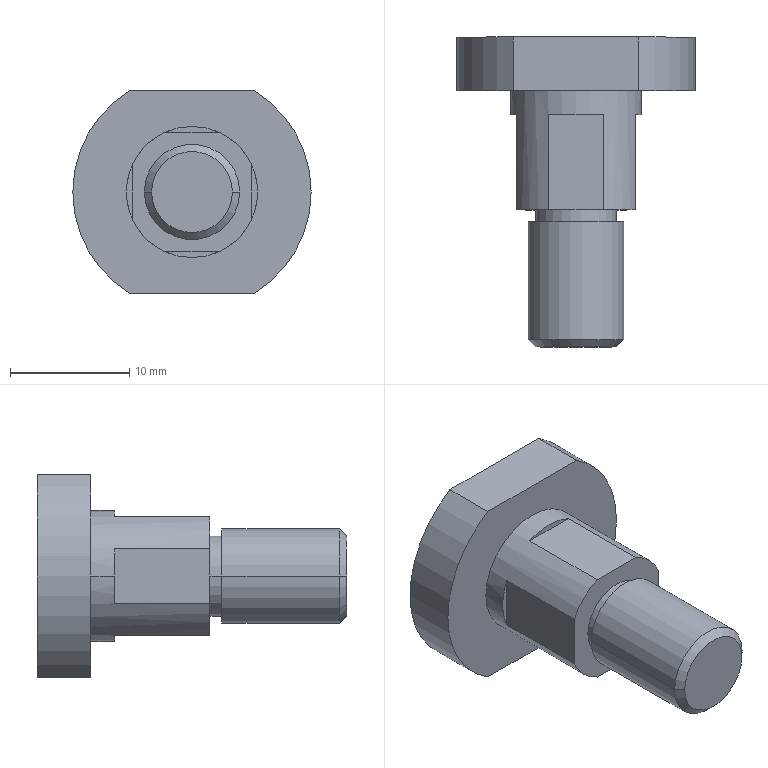Part | STEP file | BU-E02 | 1 solid | 26 faces | box 20 x 26 x 17 mm | volume 2778 mm3 | plane 15 | cylinder 9 | cone 2 | commonest cylinder face diameters 20 x3 6.8 x2 8 x2 11 x2